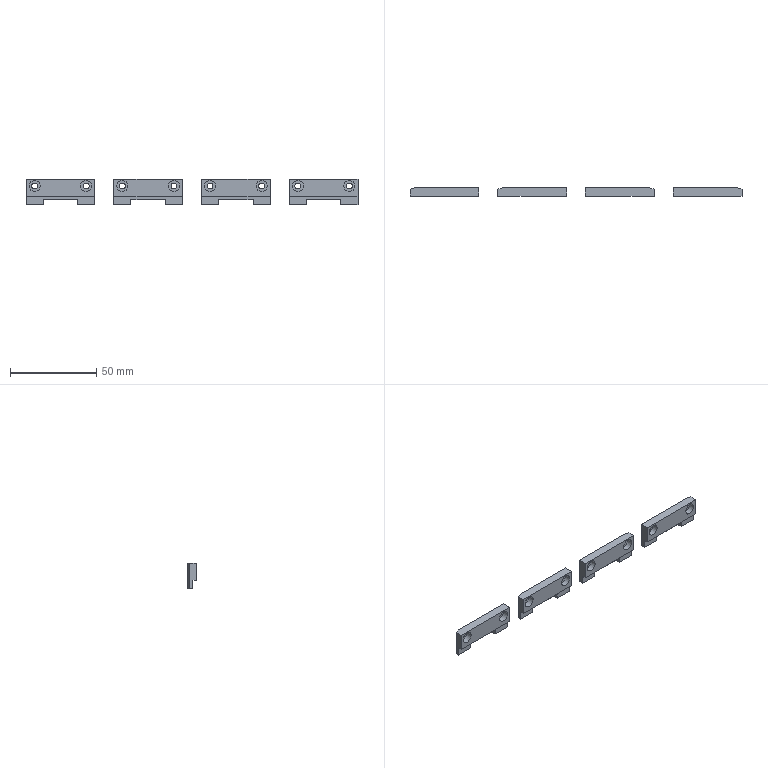Part | 4 solids | 80 faces | box 193 x 5 x 15 mm | volume 8562 mm3 | plane 64 | cylinder 16 | commonest cylinder face diameters 3.4 x8 6.5 x8